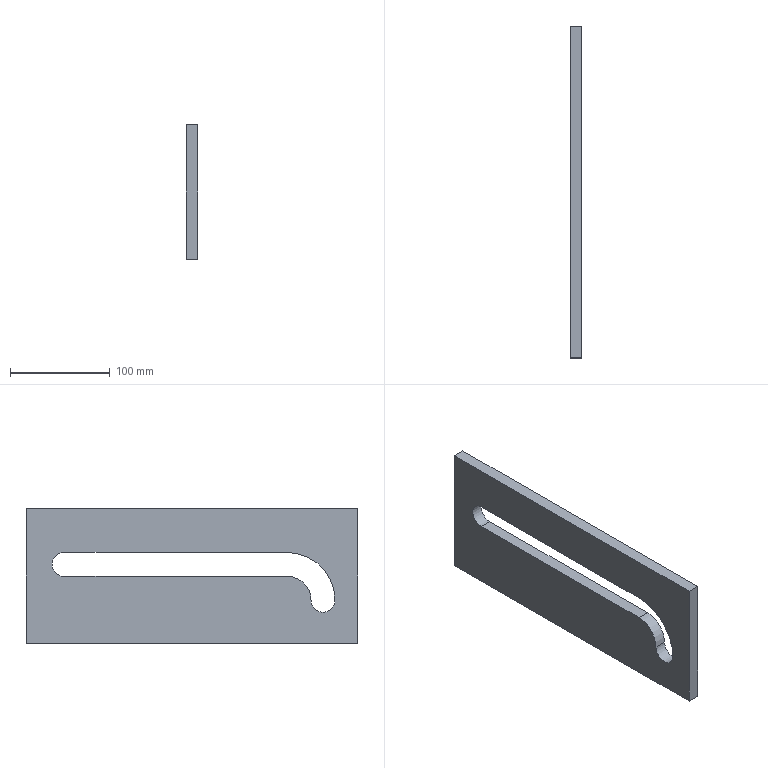Part | NX | features solid 2 | 1 solid | 12 faces | box 12 x 333 x 135 mm | volume 453234 mm3 | plane 8 | cylinder 4 | commonest cylinder face diameters 24 x2 48 x1 96 x1
STEP:
#1=CARTESIAN_POINT('',(-61.,110.3,187.866));
#2=VERTEX_POINT('',#1);
#3=CARTESIAN_POINT('',(-73.,110.3,187.866));
#4=VERTEX_POINT('',#3);
#5=CARTESIAN_POINT('',(-67.,110.3,187.866));
#6=DIRECTION('',(1.,0.,-0.000000019));
#7=VECTOR('',#6,1000.);
#8=LINE('',#5,#7);
#9=EDGE_CURVE('',#2,#4,#8,.F.);
#10=ORIENTED_EDGE('',*,*,#9,.F.);
#11=CARTESIAN_POINT('',(-61.,443.3,187.866));
#12=VERTEX_POINT('',#11);
#13=CARTESIAN_POINT('',(-61.,145.3,187.866));
#14=DIRECTION('',(0.,1.,0.));
#15=VECTOR('',#14,1000.);
#16=LINE('',#13,#15);
#17=EDGE_CURVE('',#12,#2,#16,.F.);
#18=ORIENTED_EDGE('',*,*,#17,.F.);
#19=CARTESIAN_POINT('',(-73.,443.3,187.866));
#20=VERTEX_POINT('',#19);
#21=CARTESIAN_POINT('',(-67.,443.3,187.866));
#22=DIRECTION('',(-1.,0.,0.000000019));
#23=VECTOR('',#22,1000.);
#24=LINE('',#21,#23);
#25=EDGE_CURVE('',#20,#12,#24,.F.);
#26=ORIENTED_EDGE('',*,*,#25,.F.);
#27=CARTESIAN_POINT('',(-73.,145.3,187.866));
#28=DIRECTION('',(0.,-1.,0.));
#29=VECTOR('',#28,1000.);
#30=LINE('',#27,#29);
#31=EDGE_CURVE('',#4,#20,#30,.F.);
#32=ORIENTED_EDGE('',*,*,#31,.F.);
#33=EDGE_LOOP('',(#10,#18,#26,#32));
#34=FACE_BOUND('',#33,.T.);
#35=CARTESIAN_POINT('',(58.,201.966,187.866));
#36=DIRECTION('',(-0.000000019,0.,-1.));
#37=DIRECTION('',(1.,0.,-0.000000019));
#38=AXIS2_PLACEMENT_3D('',#35,#36,#37);
#39=PLANE('',#38);
#40=ADVANCED_FACE('',(#34),#39,.F.);
#41=CARTESIAN_POINT('',(-61.,110.3,52.866));
#42=VERTEX_POINT('',#41);
#43=CARTESIAN_POINT('',(-61.,110.3,84.));
#44=DIRECTION('',(0.,0.,1.));
#45=VECTOR('',#44,1000.);
#46=LINE('',#43,#45);
#47=EDGE_CURVE('',#42,#2,#46,.T.);
#48=ORIENTED_EDGE('',*,*,#47,.T.);
#49=ORIENTED_EDGE('',*,*,#9,.T.);
#50=CARTESIAN_POINT('',(-73.,110.3,52.866));
#51=VERTEX_POINT('',#50);
#52=CARTESIAN_POINT('',(-73.,110.3,84.));
#53=DIRECTION('',(0.,0.,1.));
#54=VECTOR('',#53,1000.);
#55=LINE('',#52,#54);
#56=EDGE_CURVE('',#51,#4,#55,.T.);
#57=ORIENTED_EDGE('',*,*,#56,.F.);
#58=CARTESIAN_POINT('',(-67.,110.3,52.866));
#59=DIRECTION('',(1.,0.,0.));
#60=VECTOR('',#59,1000.);
#61=LINE('',#58,#60);
#62=EDGE_CURVE('',#51,#42,#61,.T.);
#63=ORIENTED_EDGE('',*,*,#62,.T.);
#64=EDGE_LOOP('',(#48,#49,#57,#63));
#65=FACE_BOUND('',#64,.T.);
#66=CARTESIAN_POINT('',(-67.,110.3,84.));
#67=DIRECTION('',(0.,-1.,0.));
#68=DIRECTION('',(0.,0.,-1.));
#69=AXIS2_PLACEMENT_3D('',#66,#67,#68);
#70=PLANE('',#69);
#71=ADVANCED_FACE('',(#65),#70,.T.);
#72=CARTESIAN_POINT('',(-73.,405.3,144.));
#73=VERTEX_POINT('',#72);
#74=CARTESIAN_POINT('',(-73.,405.3,120.));
#75=VERTEX_POINT('',#74);
#76=CARTESIAN_POINT('',(-73.,405.3,132.));
#77=DIRECTION('',(-1.,0.,0.));
#78=DIRECTION('',(0.,0.,1.));
#79=AXIS2_PLACEMENT_3D('',#76,#77,#78);
#80=CIRCLE('',#79,12.);
#81=EDGE_CURVE('',#73,#75,#80,.T.);
#82=ORIENTED_EDGE('',*,*,#81,.F.);
#83=CARTESIAN_POINT('',(-73.,181.3,144.));
#84=VERTEX_POINT('',#83);
#85=CARTESIAN_POINT('',(-73.,251.3,144.));
#86=DIRECTION('',(0.,-1.,0.));
#87=VECTOR('',#86,1000.);
#88=LINE('',#85,#87);
#89=EDGE_CURVE('',#84,#73,#88,.F.);
#90=ORIENTED_EDGE('',*,*,#89,.F.);
#91=CARTESIAN_POINT('',(-73.,133.3,96.));
#92=VERTEX_POINT('',#91);
#93=CARTESIAN_POINT('',(-73.,181.3,96.));
#94=DIRECTION('',(-1.,0.,0.));
#95=DIRECTION('',(0.,0.,1.));
#96=AXIS2_PLACEMENT_3D('',#93,#94,#95);
#97=CIRCLE('',#96,48.);
#98=EDGE_CURVE('',#92,#84,#97,.T.);
#99=ORIENTED_EDGE('',*,*,#98,.F.);
#100=CARTESIAN_POINT('',(-73.,157.3,96.));
#101=VERTEX_POINT('',#100);
#102=CARTESIAN_POINT('',(-73.,145.3,96.));
#103=DIRECTION('',(-1.,0.,0.));
#104=DIRECTION('',(0.,0.,1.));
#105=AXIS2_PLACEMENT_3D('',#102,#103,#104);
#106=CIRCLE('',#105,12.);
#107=EDGE_CURVE('',#101,#92,#106,.T.);
#108=ORIENTED_EDGE('',*,*,#107,.F.);
#109=CARTESIAN_POINT('',(-73.,181.3,120.));
#110=VERTEX_POINT('',#109);
#111=CARTESIAN_POINT('',(-73.,181.3,96.));
#112=DIRECTION('',(-1.,0.,0.));
#113=DIRECTION('',(0.,0.,1.));
#114=AXIS2_PLACEMENT_3D('',#111,#112,#113);
#115=CIRCLE('',#114,24.);
#116=EDGE_CURVE('',#110,#101,#115,.F.);
#117=ORIENTED_EDGE('',*,*,#116,.F.);
#118=CARTESIAN_POINT('',(-73.,251.3,120.));
#119=DIRECTION('',(0.,-1.,0.));
#120=VECTOR('',#119,1000.);
#121=LINE('',#118,#120);
#122=EDGE_CURVE('',#110,#75,#121,.F.);
#123=ORIENTED_EDGE('',*,*,#122,.T.);
#124=EDGE_LOOP('',(#82,#90,#99,#108,#117,#123));
#125=FACE_BOUND('',#124,.T.);
#126=ORIENTED_EDGE('',*,*,#56,.T.);
#127=ORIENTED_EDGE('',*,*,#31,.T.);
#128=CARTESIAN_POINT('',(-73.,443.3,52.866));
#129=VERTEX_POINT('',#128);
#130=CARTESIAN_POINT('',(-73.,443.3,84.));
#131=DIRECTION('',(0.,0.,1.));
#132=VECTOR('',#131,1000.);
#133=LINE('',#130,#132);
#134=EDGE_CURVE('',#129,#20,#133,.T.);
#135=ORIENTED_EDGE('',*,*,#134,.F.);
#136=CARTESIAN_POINT('',(-73.,145.3,52.866));
#137=DIRECTION('',(0.,-1.,0.));
#138=VECTOR('',#137,1000.);
#139=LINE('',#136,#138);
#140=EDGE_CURVE('',#129,#51,#139,.T.);
#141=ORIENTED_EDGE('',*,*,#140,.T.);
#142=EDGE_LOOP('',(#126,#127,#135,#141));
#143=FACE_BOUND('',#142,.T.);
#144=CARTESIAN_POINT('',(-73.,145.3,84.));
#145=DIRECTION('',(-1.,0.,0.));
#146=DIRECTION('',(0.,0.,1.));
#147=AXIS2_PLACEMENT_3D('',#144,#145,#146);
#148=PLANE('',#147);
#149=ADVANCED_FACE('',(#125,#143),#148,.T.);
#150=ORIENTED_EDGE('',*,*,#134,.T.);
#151=ORIENTED_EDGE('',*,*,#25,.T.);
#152=CARTESIAN_POINT('',(-61.,443.3,52.866));
#153=VERTEX_POINT('',#152);
#154=CARTESIAN_POINT('',(-61.,443.3,84.));
#155=DIRECTION('',(0.,0.,1.));
#156=VECTOR('',#155,1000.);
#157=LINE('',#154,#156);
#158=EDGE_CURVE('',#153,#12,#157,.T.);
#159=ORIENTED_EDGE('',*,*,#158,.F.);
#160=CARTESIAN_POINT('',(-67.,443.3,52.866));
#161=DIRECTION('',(-1.,0.,0.));
#162=VECTOR('',#161,1000.);
#163=LINE('',#160,#162);
#164=EDGE_CURVE('',#153,#129,#163,.T.);
#165=ORIENTED_EDGE('',*,*,#164,.T.);
#166=EDGE_LOOP('',(#150,#151,#159,#165));
#167=FACE_BOUND('',#166,.T.);
#168=CARTESIAN_POINT('',(-67.,443.3,84.));
#169=DIRECTION('',(0.,1.,0.));
#170=DIRECTION('',(0.,0.,1.));
#171=AXIS2_PLACEMENT_3D('',#168,#169,#170);
#172=PLANE('',#171);
#173=ADVANCED_FACE('',(#167),#172,.T.);
#174=CARTESIAN_POINT('',(-61.,145.3,52.866));
#175=DIRECTION('',(0.,1.,0.));
#176=VECTOR('',#175,1000.);
#177=LINE('',#174,#176);
#178=EDGE_CURVE('',#42,#153,#177,.T.);
#179=ORIENTED_EDGE('',*,*,#178,.F.);
#180=ORIENTED_EDGE('',*,*,#62,.F.);
#181=ORIENTED_EDGE('',*,*,#140,.F.);
#182=ORIENTED_EDGE('',*,*,#164,.F.);
#183=EDGE_LOOP('',(#179,#180,#181,#182));
#184=FACE_BOUND('',#183,.T.);
#185=CARTESIAN_POINT('',(-67.,145.3,52.866));
#186=DIRECTION('',(0.,0.,-1.));
#187=DIRECTION('',(-1.,0.,0.));
#188=AXIS2_PLACEMENT_3D('',#185,#186,#187);
#189=PLANE('',#188);
#190=ADVANCED_FACE('',(#184),#189,.T.);
#191=CARTESIAN_POINT('',(-61.,181.3,120.));
#192=VERTEX_POINT('',#191);
#193=CARTESIAN_POINT('',(-61.,405.3,120.));
#194=VERTEX_POINT('',#193);
#195=CARTESIAN_POINT('',(-61.,251.3,120.));
#196=DIRECTION('',(0.,-1.,0.));
#197=VECTOR('',#196,1000.);
#198=LINE('',#195,#197);
#199=EDGE_CURVE('',#192,#194,#198,.F.);
#200=ORIENTED_EDGE('',*,*,#199,.F.);
#201=CARTESIAN_POINT('',(-61.,157.3,96.));
#202=VERTEX_POINT('',#201);
#203=CARTESIAN_POINT('',(-61.,181.3,96.));
#204=DIRECTION('',(1.,0.,0.));
#205=DIRECTION('',(0.,0.,-1.));
#206=AXIS2_PLACEMENT_3D('',#203,#204,#205);
#207=CIRCLE('',#206,24.);
#208=EDGE_CURVE('',#202,#192,#207,.F.);
#209=ORIENTED_EDGE('',*,*,#208,.F.);
#210=CARTESIAN_POINT('',(-61.,133.3,96.));
#211=VERTEX_POINT('',#210);
#212=CARTESIAN_POINT('',(-61.,145.3,96.));
#213=DIRECTION('',(1.,0.,0.));
#214=DIRECTION('',(0.,0.,-1.));
#215=AXIS2_PLACEMENT_3D('',#212,#213,#214);
#216=CIRCLE('',#215,12.);
#217=EDGE_CURVE('',#211,#202,#216,.T.);
#218=ORIENTED_EDGE('',*,*,#217,.F.);
#219=CARTESIAN_POINT('',(-61.,181.3,144.));
#220=VERTEX_POINT('',#219);
#221=CARTESIAN_POINT('',(-61.,181.3,96.));
#222=DIRECTION('',(1.,0.,0.));
#223=DIRECTION('',(0.,0.,-1.));
#224=AXIS2_PLACEMENT_3D('',#221,#222,#223);
#225=CIRCLE('',#224,48.);
#226=EDGE_CURVE('',#220,#211,#225,.T.);
#227=ORIENTED_EDGE('',*,*,#226,.F.);
#228=CARTESIAN_POINT('',(-61.,405.3,144.));
#229=VERTEX_POINT('',#228);
#230=CARTESIAN_POINT('',(-61.,251.3,144.));
#231=DIRECTION('',(0.,-1.,0.));
#232=VECTOR('',#231,1000.);
#233=LINE('',#230,#232);
#234=EDGE_CURVE('',#229,#220,#233,.T.);
#235=ORIENTED_EDGE('',*,*,#234,.F.);
#236=CARTESIAN_POINT('',(-61.,405.3,132.));
#237=DIRECTION('',(1.,0.,0.));
#238=DIRECTION('',(0.,0.,-1.));
#239=AXIS2_PLACEMENT_3D('',#236,#237,#238);
#240=CIRCLE('',#239,12.);
#241=EDGE_CURVE('',#194,#229,#240,.T.);
#242=ORIENTED_EDGE('',*,*,#241,.F.);
#243=EDGE_LOOP('',(#200,#209,#218,#227,#235,#242));
#244=FACE_BOUND('',#243,.T.);
#245=ORIENTED_EDGE('',*,*,#178,.T.);
#246=ORIENTED_EDGE('',*,*,#158,.T.);
#247=ORIENTED_EDGE('',*,*,#17,.T.);
#248=ORIENTED_EDGE('',*,*,#47,.F.);
#249=EDGE_LOOP('',(#245,#246,#247,#248));
#250=FACE_BOUND('',#249,.T.);
#251=CARTESIAN_POINT('',(-61.,145.3,84.));
#252=DIRECTION('',(1.,0.,0.));
#253=DIRECTION('',(0.,0.,-1.));
#254=AXIS2_PLACEMENT_3D('',#251,#252,#253);
#255=PLANE('',#254);
#256=ADVANCED_FACE('',(#244,#250),#255,.T.);
#257=ORIENTED_EDGE('',*,*,#234,.T.);
#258=CARTESIAN_POINT('',(-67.,181.3,144.));
#259=DIRECTION('',(-1.,0.,0.));
#260=VECTOR('',#259,1000.);
#261=LINE('',#258,#260);
#262=EDGE_CURVE('',#220,#84,#261,.T.);
#263=ORIENTED_EDGE('',*,*,#262,.T.);
#264=ORIENTED_EDGE('',*,*,#89,.T.);
#265=CARTESIAN_POINT('',(-67.,405.3,144.));
#266=DIRECTION('',(-1.,0.,0.));
#267=VECTOR('',#266,1000.);
#268=LINE('',#265,#267);
#269=EDGE_CURVE('',#73,#229,#268,.F.);
#270=ORIENTED_EDGE('',*,*,#269,.T.);
#271=EDGE_LOOP('',(#257,#263,#264,#270));
#272=FACE_BOUND('',#271,.T.);
#273=CARTESIAN_POINT('',(-67.,251.3,144.));
#274=DIRECTION('',(0.,0.,1.));
#275=DIRECTION('',(0.,1.,0.));
#276=AXIS2_PLACEMENT_3D('',#273,#274,#275);
#277=PLANE('',#276);
#278=ADVANCED_FACE('',(#272),#277,.F.);
#279=ORIENTED_EDGE('',*,*,#122,.F.);
#280=CARTESIAN_POINT('',(-73.,181.3,120.));
#281=DIRECTION('',(1.,0.,0.));
#282=VECTOR('',#281,1000.);
#283=LINE('',#280,#282);
#284=EDGE_CURVE('',#110,#192,#283,.T.);
#285=ORIENTED_EDGE('',*,*,#284,.T.);
#286=ORIENTED_EDGE('',*,*,#199,.T.);
#287=CARTESIAN_POINT('',(-67.,405.3,120.));
#288=DIRECTION('',(1.,0.,0.));
#289=VECTOR('',#288,1000.);
#290=LINE('',#287,#289);
#291=EDGE_CURVE('',#194,#75,#290,.F.);
#292=ORIENTED_EDGE('',*,*,#291,.T.);
#293=EDGE_LOOP('',(#279,#285,#286,#292));
#294=FACE_BOUND('',#293,.T.);
#295=CARTESIAN_POINT('',(-67.,251.3,120.));
#296=DIRECTION('',(0.,0.,-1.));
#297=DIRECTION('',(0.,-1.,0.));
#298=AXIS2_PLACEMENT_3D('',#295,#296,#297);
#299=PLANE('',#298);
#300=ADVANCED_FACE('',(#294),#299,.F.);
#301=ORIENTED_EDGE('',*,*,#217,.T.);
#302=CARTESIAN_POINT('',(-67.,157.3,96.));
#303=DIRECTION('',(-1.,0.,0.));
#304=VECTOR('',#303,1000.);
#305=LINE('',#302,#304);
#306=EDGE_CURVE('',#101,#202,#305,.F.);
#307=ORIENTED_EDGE('',*,*,#306,.F.);
#308=ORIENTED_EDGE('',*,*,#107,.T.);
#309=CARTESIAN_POINT('',(-67.,133.3,96.));
#310=DIRECTION('',(1.,0.,0.));
#311=VECTOR('',#310,1000.);
#312=LINE('',#309,#311);
#313=EDGE_CURVE('',#211,#92,#312,.F.);
#314=ORIENTED_EDGE('',*,*,#313,.F.);
#315=EDGE_LOOP('',(#301,#307,#308,#314));
#316=FACE_BOUND('',#315,.T.);
#317=CARTESIAN_POINT('',(-67.,145.3,96.));
#318=DIRECTION('',(-1.,0.,0.));
#319=DIRECTION('',(0.,0.,1.));
#320=AXIS2_PLACEMENT_3D('',#317,#318,#319);
#321=CYLINDRICAL_SURFACE('',#320,12.);
#322=ADVANCED_FACE('',(#316),#321,.F.);
#323=ORIENTED_EDGE('',*,*,#116,.T.);
#324=ORIENTED_EDGE('',*,*,#306,.T.);
#325=ORIENTED_EDGE('',*,*,#208,.T.);
#326=ORIENTED_EDGE('',*,*,#284,.F.);
#327=EDGE_LOOP('',(#323,#324,#325,#326));
#328=FACE_BOUND('',#327,.T.);
#329=CARTESIAN_POINT('',(-67.,181.3,96.));
#330=DIRECTION('',(-1.,0.,0.));
#331=DIRECTION('',(0.,0.,1.));
#332=AXIS2_PLACEMENT_3D('',#329,#330,#331);
#333=CYLINDRICAL_SURFACE('',#332,24.);
#334=ADVANCED_FACE('',(#328),#333,.T.);
#335=ORIENTED_EDGE('',*,*,#226,.T.);
#336=ORIENTED_EDGE('',*,*,#313,.T.);
#337=ORIENTED_EDGE('',*,*,#98,.T.);
#338=ORIENTED_EDGE('',*,*,#262,.F.);
#339=EDGE_LOOP('',(#335,#336,#337,#338));
#340=FACE_BOUND('',#339,.T.);
#341=CARTESIAN_POINT('',(-67.,181.3,96.));
#342=DIRECTION('',(-1.,0.,0.));
#343=DIRECTION('',(0.,0.,1.));
#344=AXIS2_PLACEMENT_3D('',#341,#342,#343);
#345=CYLINDRICAL_SURFACE('',#344,48.);
#346=ADVANCED_FACE('',(#340),#345,.F.);
#347=ORIENTED_EDGE('',*,*,#241,.T.);
#348=ORIENTED_EDGE('',*,*,#269,.F.);
#349=ORIENTED_EDGE('',*,*,#81,.T.);
#350=ORIENTED_EDGE('',*,*,#291,.F.);
#351=EDGE_LOOP('',(#347,#348,#349,#350));
#352=FACE_BOUND('',#351,.T.);
#353=CARTESIAN_POINT('',(-67.,405.3,132.));
#354=DIRECTION('',(-1.,0.,0.));
#355=DIRECTION('',(0.,0.,1.));
#356=AXIS2_PLACEMENT_3D('',#353,#354,#355);
#357=CYLINDRICAL_SURFACE('',#356,12.);
#358=ADVANCED_FACE('',(#352),#357,.F.);
#359=CLOSED_SHELL('',(#40,#71,#149,#173,#190,#256,#278,#300,#322,#334,#346,#358));
#360=MANIFOLD_SOLID_BREP('',#359);
#361=(LENGTH_UNIT()NAMED_UNIT(*)SI_UNIT(.MILLI.,.METRE.));
#362=UNCERTAINTY_MEASURE_WITH_UNIT(LENGTH_MEASURE(0.00001),#361,'','');
#363=(NAMED_UNIT(*)PLANE_ANGLE_UNIT()SI_UNIT($,.RADIAN.));
#364=(NAMED_UNIT(*)SI_UNIT($,.STERADIAN.)SOLID_ANGLE_UNIT());
#365=(GEOMETRIC_REPRESENTATION_CONTEXT(3)GLOBAL_UNCERTAINTY_ASSIGNED_CONTEXT((#362))GLOBAL_UNIT_ASSIGNED_CONTEXT((#361,#363,#364))REPRESENTATION_CONTEXT('',''));
#366=ADVANCED_BREP_SHAPE_REPRESENTATION('',(#360),#365);